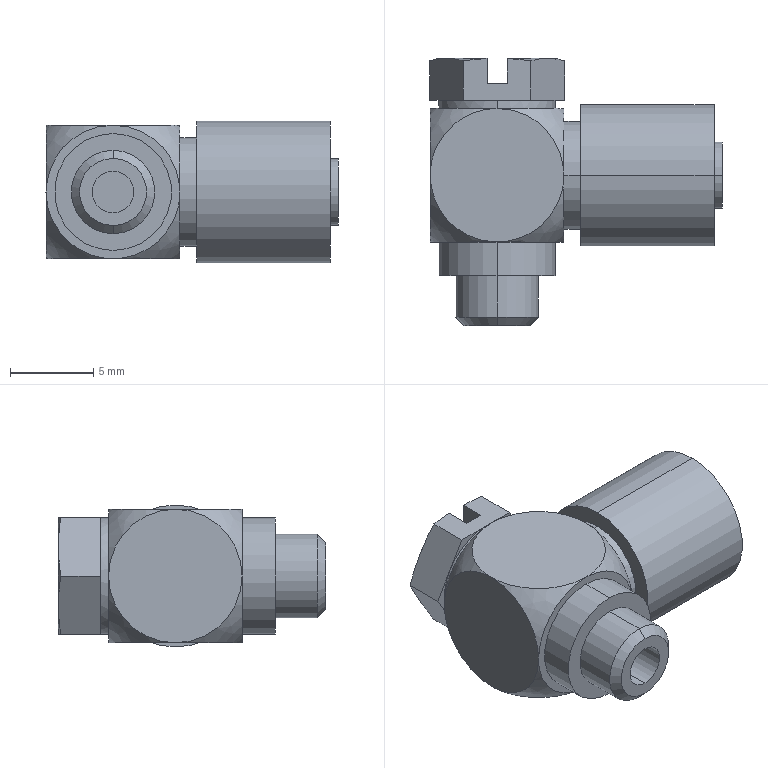Part | STEP file | M-5HLH-6 | 1 solid | 62 faces | box 17.541 x 16 x 8.5 mm | volume 1152 mm3 | plane 30 | cylinder 16 | cone 8 | spline 8 | commonest cylinder face diameters 2.5 x4 7 x4 4 x2 5 x2 6.5 x2 8.5 x2